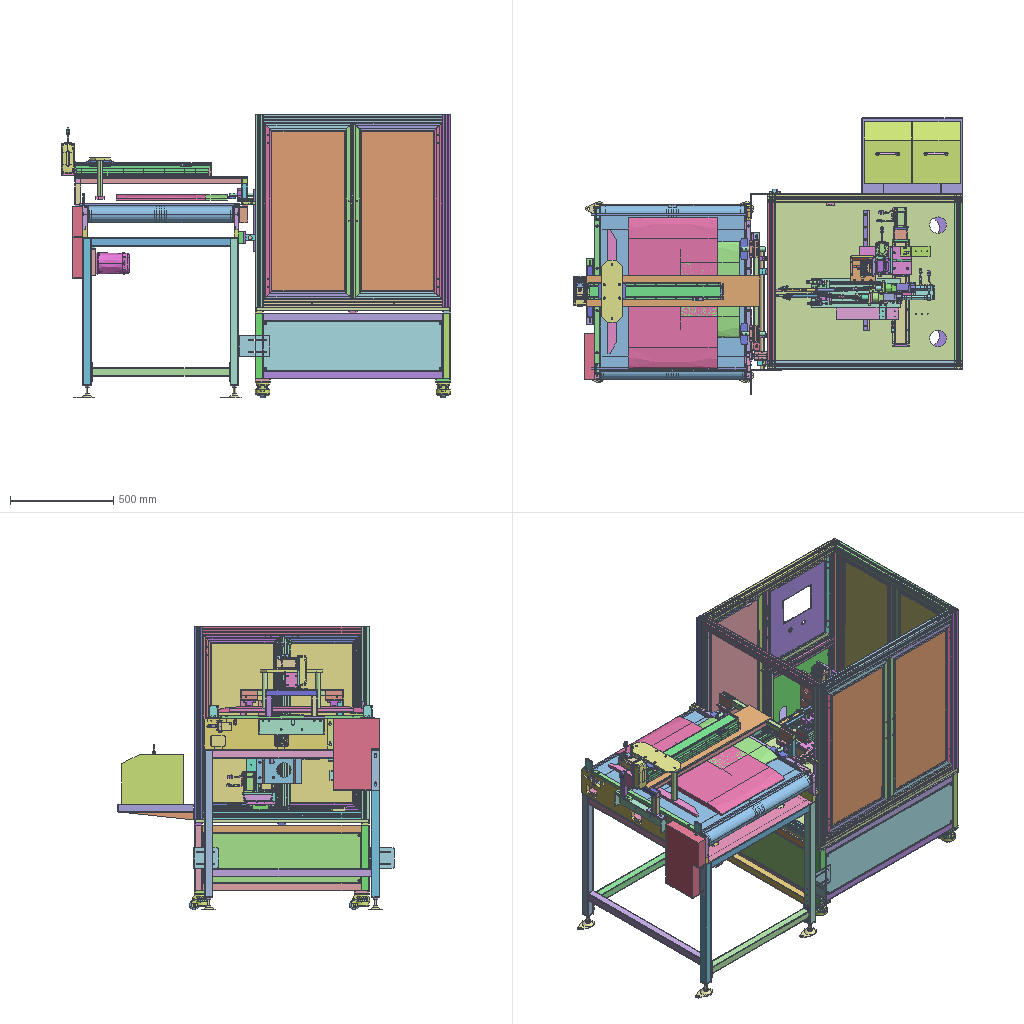Assembly | SolidWorks | 110 different items | 141 placed | box 1890 x 1340 x 1377 mm
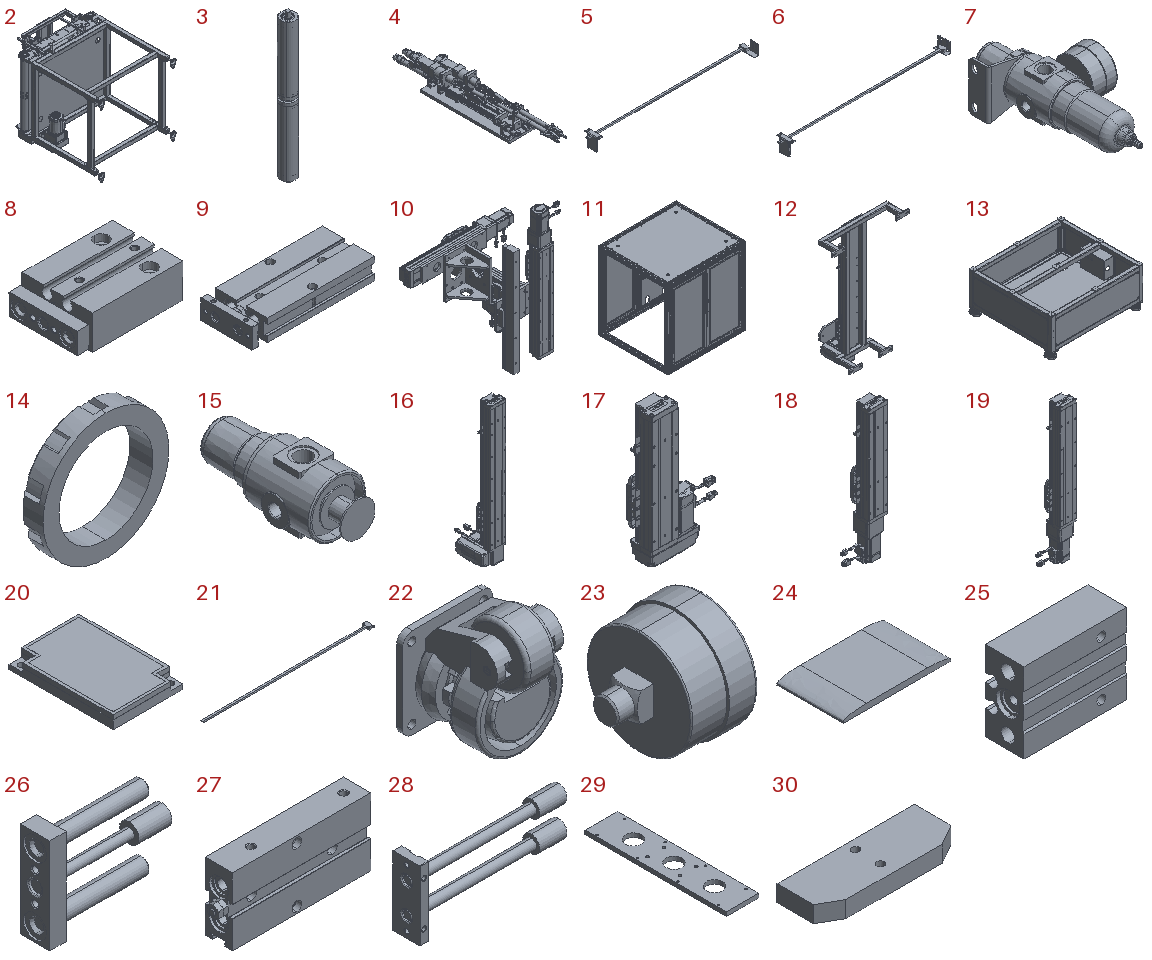Parts list (item | name | quantity | parent item | size | volume | features):
1 | (subassembly) | x1 | - | - | - | features Attribute 54, InContextFeatHolder 18
2 | (subassembly) | x1 | - | - | 25748774 mm3 | features ReferencePattern 2, CompositeCurve 1, MirrorCompFeat 1
3 | (subassembly) | x1 | in 2 | 76 x 76 x 755 mm | 913977 mm3 | features MirrorCompFeat 1
4 | (subassembly) | x1 | in 1 | - | 1977709 mm3 | -
5 | (subassembly) | x1 | in 2 | 779.985 x 90 x 92.8 mm | 90208 mm3 | -
6 | (subassembly) | x1 | in 2 | 779.985 x 68 x 92.8 mm | 89930 mm3 | -
7 | (subassembly) | x1 | in 13 | 87.334 x 158 x 50 mm | 129441 mm3 | features AEMSimFeature 1
8 | (subassembly) | x1 | in 2 | 44.5 x 30 x 14.5 mm | 15522 mm3 | features AEMSimFeature 1
9 | (subassembly) | x1 | in 2 | 98 x 42 x 17 mm | 52480 mm3 | features AEMSimFeature 1
10 | (subassembly) | x1 | in 1 | - | 10894817 mm3 | features InContextFeatHolder 20
11 | (subassembly) | x1 | - | - | 21354940 mm3 | -
12 | (subassembly) | x1 | in 2 | 570 x 381.182 x 905.5 mm | 5879539 mm3 | features ReferencePattern 4, InContextFeatHolder 2, MirrorCompFeat 1
13 | (subassembly) | x1 | - | 950 x 876 x 421.5 mm | 6731533 mm3 | features InContextFeatHolder 11, CompositeCurve 1
14 | - | x1 | in 7 | 38 x 7 x 38 mm | 3168 mm3 | features BaseBody 1
15 | - | x1 | in 7 | 40 x 98.3 x 40 mm | 76499 mm3 | features BaseBody 1
16 | - | x1 | in 12 | - | - | features BaseBody 15, RefSurface 8
17 | - | x1 | in 10 | - | - | features BaseBody 16, RefSurface 6
18 | - | x1 | in 10 | - | - | features BaseBody 14, RefSurface 8
19 | - | x2 | in 1, 10 | - | - | features BaseBody 14, RefSurface 8
20 | - | x2 | in 5, 6 | 40.3 x 59.9 x 7.5 mm | 17477 mm3 | features BaseBody 1
21 | - | x2 | in 5, 6 | 779.985 x 38.085 x 10.8 mm | 59248 mm3 | features BaseBody 1, ICE 1
22 | - | x4 | in 13 | 73 x 81.5 x 99 mm | 238657 mm3 | features BaseBody 4
23 | - | x1 | in 7 | 37.5 x 42 x 42 mm | 32291 mm3 | features BaseBody 1
24 | - | x1 | - | 465 x 285 x 25.029 mm | 3079068 mm3 | features Fillet 2, Extrusion 1
25 | - | x1 | in 8 | 38.5 x 14.5 x 30 mm | 12801 mm3 | features BaseBody 1
26 | - | x1 | in 8 | 38.7 x 9 x 29 mm | 2721 mm3 | features BaseBody 1
27 | - | x1 | in 9 | 93 x 17 x 42 mm | 43135 mm3 | features BaseBody 1
28 | - | x1 | in 9 | 90.1 x 16 x 41 mm | 9345 mm3 | features BaseBody 1
29 | - | x1 | in 10 | 80 x 350 x 10 mm | 238170 mm3 | features HoleWzd 2, Extrusion 1, ICE 1, LPattern 1
30 | - | x2 | in 12 | 100 x 35 x 12 mm | 39246 mm3 | features Chamfer 1, Extrusion 1, HoleWzd 1
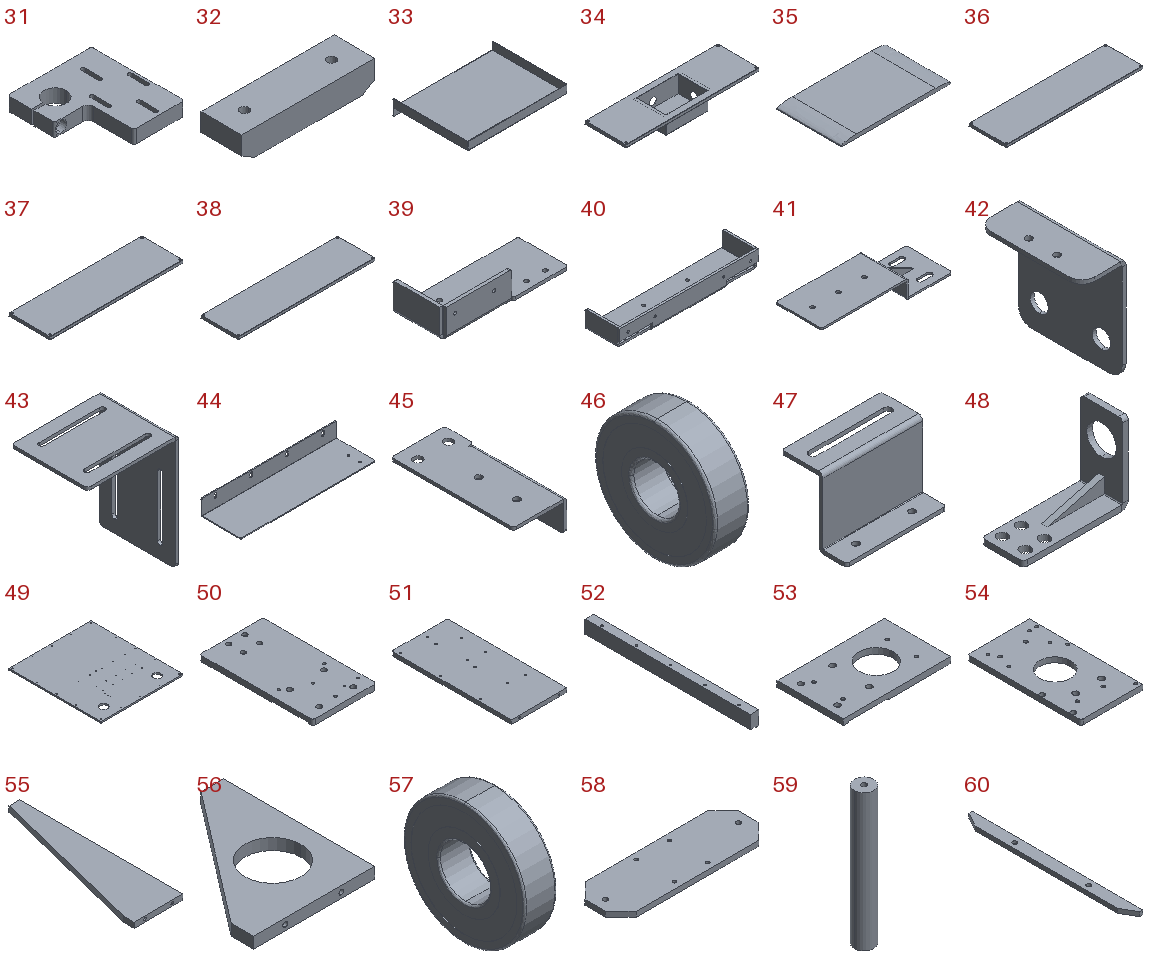31 | - | x1 | in 2 | 75 x 83 x 12 mm | 51875 mm3 | features ICE 4, HoleWzd 3, Fillet 2, LPattern 2, Extrusion 1, MoveFace 1
32 | - | x1 | in 2 | 52 x 16 x 10 mm | 7777 mm3 | features Chamfer 2, Extrusion 1, HoleWzd 1
33 | - | x1 | - | 490 x 370 x 77 mm | 765884 mm3 | features Gusset 2, EdgeFlange 1, Fillet 1, FlatPattern 1, HoleWzd 1, SMBaseFlange 1, SheetMetal 1
34 | - | x1 | in 13 | 768 x 238 x 101.5 mm | 482103 mm3 | features EdgeFlange 4, Cut 3, FlatPattern 2, HoleWzd 2, SMBaseFlange 2, SheetMetal 2, ICE 1
35 | - | x1 | - | 730 x 430 x 25.029 mm | 7503443 mm3 | features Fillet 2, Extrusion 1
36 | - | x1 | in 13 | 868 x 238 x 17.5 mm | 401918 mm3 | features EdgeFlange 2, Cut 1, FlatPattern 1, HoleWzd 1, SMBaseFlange 1, SheetMetal 1
37 | - | x1 | in 13 | 768 x 238 x 17.5 mm | 357698 mm3 | features EdgeFlange 2, Cut 1, FlatPattern 1, HoleWzd 1, SMBaseFlange 1, SheetMetal 1
38 | - | x1 | in 13 | 868 x 238 x 17.5 mm | 401918 mm3 | features EdgeFlange 2, Cut 1, FlatPattern 1, HoleWzd 1, SMBaseFlange 1, SheetMetal 1
39 | - | x1 | in 2 | 200 x 80 x 45 mm | 113530 mm3 | features HoleWzd 3, EdgeFlange 1, Fillet 1, FlatPattern 1, SMBaseFlange 1, SheetMetal 1
40 | - | x1 | in 2 | 320 x 80 x 40 mm | 194537 mm3 | features HoleWzd 3, MoveFace 2, EdgeFlange 1, Fillet 1, FlatPattern 1, ICE 1, MirrorPattern 1, SMBaseFlange 1, SheetMetal 1
41 | - | x1 | in 1 | 143 x 50 x 20 mm | 15978 mm3 | features EdgeFlange 2, Fillet 1, FlatPattern 1, Gusset 1, HoleWzd 1, ICE 1, SMBaseFlange 1, SheetMetal 1
42 | - | x1 | in 11 | 17 x 40 x 40 mm | 3135 mm3 | features HoleWzd 2, EdgeFlange 1, Fillet 1, FlatPattern 1, SMBaseFlange 1, SheetMetal 1
43 | - | x2 | - | 120 x 100 x 150 mm | 96309 mm3 | features ICE 2, EdgeFlange 1, Fillet 1, FlatPattern 1, SMBaseFlange 1, SheetMetal 1
44 | - | x1 | in 1 | 300 x 89 x 35 mm | 72285 mm3 | features EdgeFlange 1, Fillet 1, FlatPattern 1, HoleWzd 1, ICE 1, LPattern 1, SMBaseFlange 1, SheetMetal 1
45 | - | x1 | in 1 | 35 x 80 x 20 mm | 7504 mm3 | features HoleWzd 2, EdgeFlange 1, Fillet 1, FlatPattern 1, SMBaseFlange 1, SheetMetal 1
46 | - | x2 | in 3 | 15 x 52 x 52 mm | 19134 mm3 | features BaseBody 13
47 | - | x2 | in 12 | 80 x 52 x 56 mm | 23390 mm3 | features EdgeFlange 2, Fillet 1, FlatPattern 1, HoleWzd 1, ICE 1, SMBaseFlange 1, SheetMetal 1
48 | - | x1 | - | 55 x 22 x 42 mm | 5646 mm3 | features EdgeFlange 1, Fillet 1, FlatPattern 1, Gusset 1, HoleWzd 1, ICE 1, LPattern 1, SMBaseFlange 1, SheetMetal 1
49 | - | x1 | in 1 | 850 x 950 x 15 mm | 11946510 mm3 | features HoleWzd 5, Cut 1, Extrusion 1, Fillet 1, LPattern 1
50 | - | x1 | in 10 | 140 x 250 x 12 mm | 389185 mm3 | features HoleWzd 5, Extrusion 1, Fillet 1, ICE 1
51 | - | x1 | in 10 | 140 x 300 x 10 mm | 417191 mm3 | features HoleWzd 4, Extrusion 1, Fillet 1
52 | - | x1 | in 10 | 30 x 580 x 48 mm | 800287 mm3 | features HoleWzd 2, LPattern 2, Extrusion 1, ICE 1
53 | - | x1 | in 10 | 220 x 135 x 12 mm | 281633 mm3 | features HoleWzd 4, ICE 2, Extrusion 1
54 | - | x1 | in 10 | 120 x 220 x 10 mm | 227637 mm3 | features HoleWzd 5, Extrusion 1, Fillet 1, ICE 1
55 | - | x1 | in 10 | 90 x 300 x 10 mm | 171179 mm3 | features HoleWzd 2, Extrusion 1, ICE 1
56 | - | x4 | in 1, 10 | 108 x 135 x 10 mm | 74855 mm3 | features HoleWzd 2, ICE 2, Extrusion 1
57 | - | x2 | in 2 | 19 x 72 x 72 mm | 45746 mm3 | features BaseBody 14
58 | - | x1 | in 12 | 300 x 100 x 10 mm | 277705 mm3 | features HoleWzd 2, Chamfer 1, Extrusion 1
59 | - | x2 | in 2 | 25 x 25 x 176 mm | 84910 mm3 | features HoleWzd 2, Extrusion 1
60 | - | x1 | in 2 | 40 x 600 x 15 mm | 334405 mm3 | features Chamfer 1, Extrusion 1, HoleWzd 1
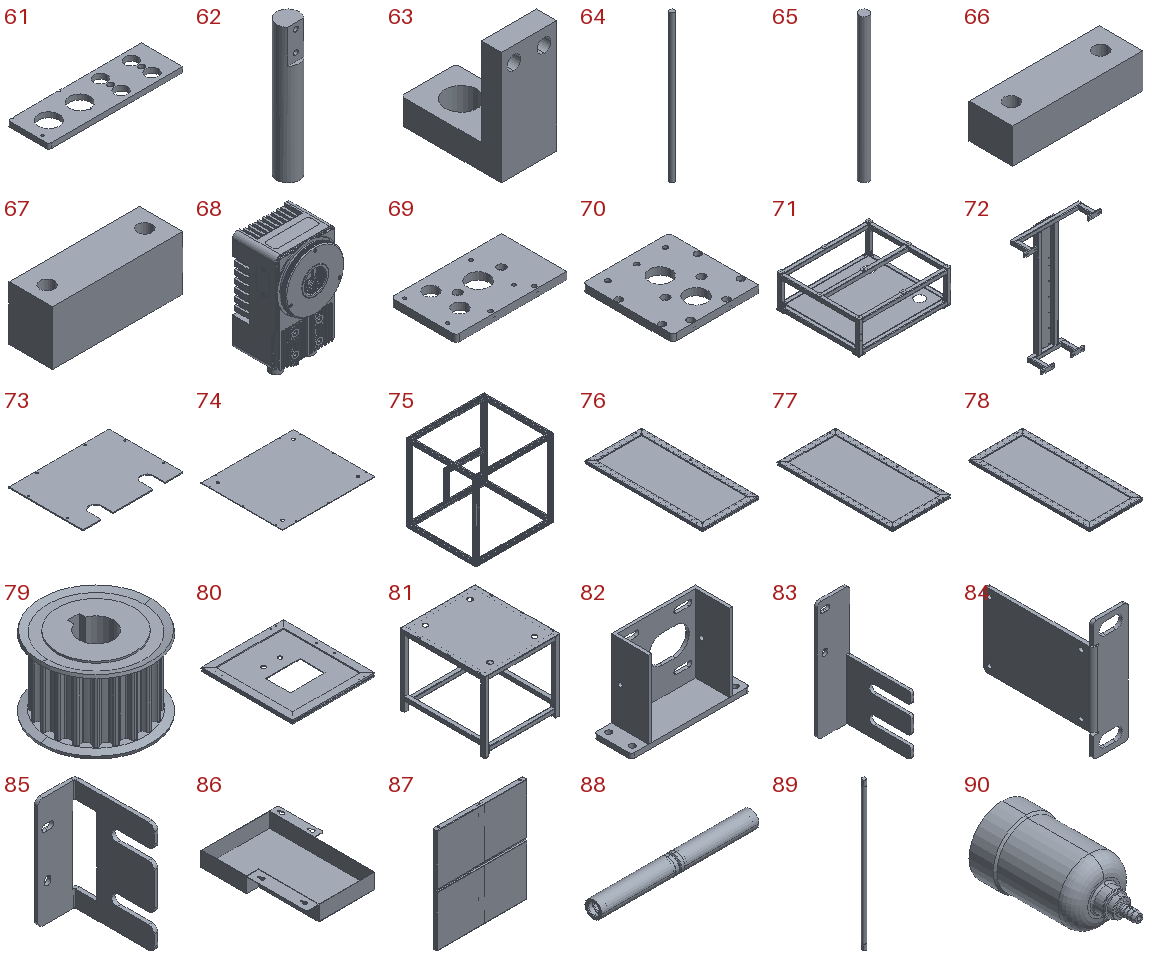61 | - | x1 | in 1 | 260 x 80 x 10 mm | 160429 mm3 | features HoleWzd 3, ICE 2, Extrusion 1, Fillet 1
62 | - | x2 | in 12 | 20 x 20 x 120 mm | 36039 mm3 | features HoleWzd 2, Extrusion 1, ICE 1
63 | - | x2 | - | 22 x 40 x 45 mm | 13243 mm3 | features BaseBody 1, ICE 1, MoveFace 1
64 | - | x1 | in 2 | 20 x 20 x 600 mm | 188496 mm3 | features Extrusion 1
65 | - | x2 | in 2 | 20 x 20 x 300 mm | 94248 mm3 | features Extrusion 1
66 | - | x1 | in 2 | 30 x 10 x 8 mm | 2124 mm3 | features Extrusion 1, HoleWzd 1
67 | - | x1 | in 2 | 60 x 20 x 25 mm | 28289 mm3 | features Extrusion 1, HoleWzd 1
68 | - | x1 | in 1 | - | - | features MBimport 1
69 | - | x1 | in 1 | 152 x 90 x 10 mm | 118972 mm3 | features HoleWzd 4, MoveFace 2, Extrusion 1, Fillet 1, ICE 1
70 | - | x1 | in 1 | 120 x 125 x 10 mm | 128886 mm3 | features HoleWzd 4, Fillet 2, ICE 2, Extrusion 1, MirrorPattern 1
71 | - | x1 | in 13 | 950 x 850 x 340 mm | 4003537 mm3 | features Fillet 10, Gusset 8, HoleWzd 8, WeldCornerFeat 8, MirrorSolid 4, ICE 3, 3DProfileFeature 1, EdgeFlange 1, FlatPattern 1, MirrorPattern 1, SMBaseFlange 1, SheetMetal 1, WeldMemberFeat 1, WeldmentFeature 1
72 | - | x1 | in 12 | 570 x 146 x 840 mm | 1678551 mm3 | features Fillet 4, ICE 4, 3DProfileFeature 1, EndCap 1, HoleWzd 1, MirrorPattern 1, WeldMemberFeat 1, WeldmentFeature 1
73 | - | x1 | in 11 | 416 x 308 x 4 mm | 483707 mm3 | features Fillet 2, HoleWzd 2, MirrorPattern 2, Extrusion 1, ICE 1
74 | - | x1 | in 11 | 868 x 768 x 4 mm | 2656781 mm3 | features MirrorPattern 4, HoleWzd 2, Extrusion 1, Fillet 1, ICE 1
75 | - | x1 | in 11 | 950 x 850 x 940 mm | 5673815 mm3 | features WeldCornerFeat 8, 3DProfileFeature 5, HoleWzd 4, ICE 1, WeldMemberFeat 1, WeldmentFeature 1
76 | - | x1 | in 11 | 407 x 856 x 20 mm | 2220771 mm3 | features HoleWzd 3, ICE 1, WeldMemberFeat 1, WeldmentFeature 1
77 | - | x2 | in 11 | 432 x 856 x 20 mm | 2324012 mm3 | features HoleWzd 3, ICE 1, WeldMemberFeat 1, WeldmentFeature 1
78 | - | x2 | in 11 | 382 x 856 x 20 mm | 2117530 mm3 | features HoleWzd 3, ICE 1, WeldMemberFeat 1, WeldmentFeature 1
79 | - | x2 | in 2 | 58 x 58 x 38.085 mm | 55625 mm3 | features BaseBody 1, ICE 1
80 | - | x1 | in 11 | 456 x 508 x 20 mm | 1433646 mm3 | features HoleWzd 3, ICE 3, WeldMemberFeat 1, WeldmentFeature 1
81 | - | x1 | in 2 | 755 x 850 x 720 mm | 5913243 mm3 | features ICE 14, Fillet 3, Cut 1, Extrusion 1, LPattern 1
82 | - | x1 | in 2 | 190 x 60 x 132 mm | 223205 mm3 | features ICE 3, Cut 1, Extrusion 1, Fillet 1
83 | - | x1 | in 5 | 22 x 45 x 80 mm | 6161 mm3 | features ICE 4, Fillet 2, ExtruThin 1, FlatPattern 1, FlattenBends 1, ProcessBends 1, SheetMetal 1
84 | - | x2 | in 5, 6 | 20 x 62 x 68 mm | 7322 mm3 | features ICE 4, Cut 1, ExtruThin 1, Fillet 1, FlatPattern 1, FlattenBends 1, ProcessBends 1, SheetMetal 1
85 | - | x1 | in 6 | 22 x 45 x 60 mm | 5883 mm3 | features Fillet 2, ICE 2, Cut 1, ExtruThin 1, FlatPattern 1, FlattenBends 1, ProcessBends 1, SheetMetal 1
86 | - | x1 | in 2 | 255 x 350 x 50 mm | 207064 mm3 | features Fillet 2, ICE 2, Cut 1, Extrusion 1, Shell 1
87 | - | x1 | in 2 | 620 x 30 x 714 mm | 1123821 mm3 | features ICE 4, BossThin 2, Extrusion 1, Fillet 1, FlatPattern 1, FlattenBends 1, LPattern 1, ProcessBends 1, Rip 1, SheetMetal 1, Shell 1
88 | - | x1 | in 3 | 705 x 76 x 76 mm | 640493 mm3 | features ICE 3, RevCut 2, Revolution 2, MirrorPattern 1
89 | - | x1 | in 3 | 20 x 20 x 755 mm | 235219 mm3 | features ICE 2, Extrusion 1, MirrorPattern 1
90 | - | x1 | in 7 | 35.6 x 74 x 35.6 mm | 13537 mm3 | features BaseBody 1
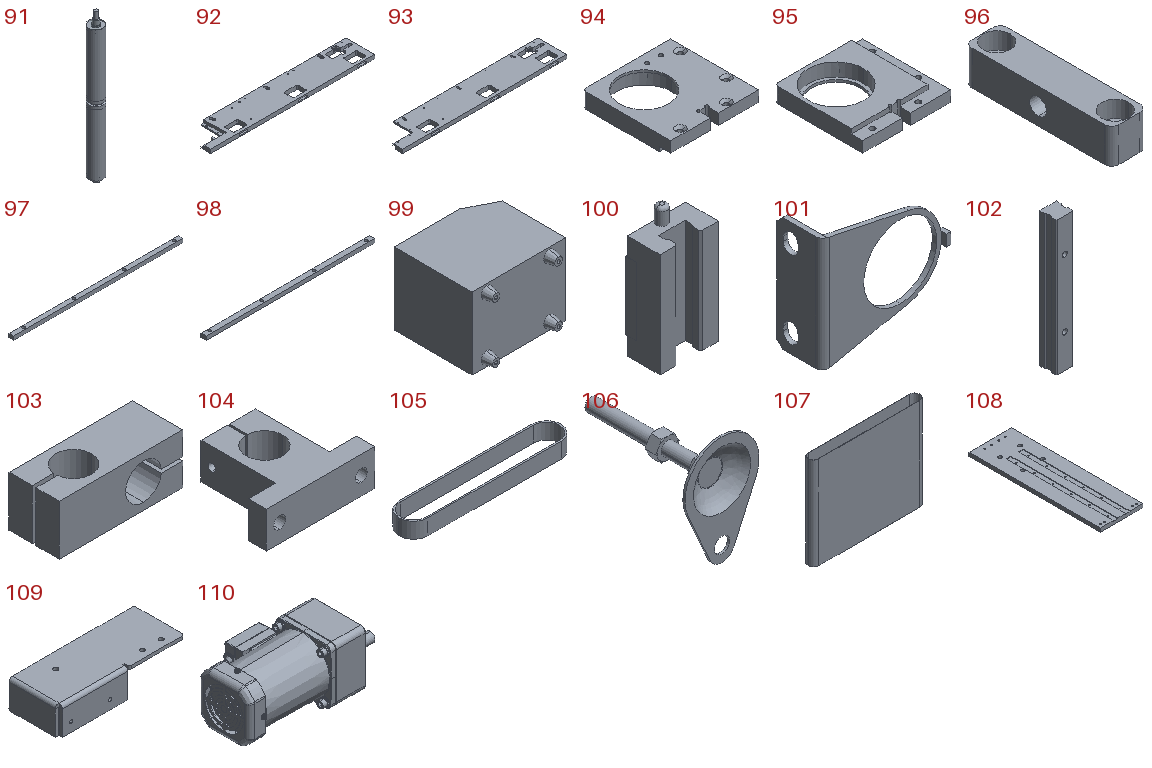91 | - | x1 | in 2 | 76 x 76 x 795 mm | 1220082 mm3 | features ICE 9, Extrusion 1, RevCut 1, Revolution 1
92 | - | x1 | in 2 | 850 x 150 x 20 mm | 1984995 mm3 | features HoleWzd 7, ICE 6, Fillet 4, Cut 1, Extrusion 1, LPattern 1
93 | - | x1 | in 2 | 850 x 150 x 20 mm | 1984995 mm3 | features MirrorStock 1
94 | - | x1 | in 2 | 115 x 115 x 20 mm | 159742 mm3 | features ICE 5, HoleWzd 3, Extrusion 1, Fillet 1
95 | - | x1 | in 2 | 115 x 115 x 20 mm | 159742 mm3 | features MirrorStock 1
96 | - | x2 | in 2 | 14.5 x 59.5 x 14 mm | 9659 mm3 | features HoleWzd 2, Extrusion 1, Fillet 1
97 | - | x1 | in 2 | 690 x 20 x 15 mm | 203293 mm3 | features Extrusion 1, HoleWzd 1, ICE 1
98 | - | x1 | in 2 | 665 x 20 x 15 mm | 195793 mm3 | features Extrusion 1, HoleWzd 1
99 | - | x2 | - | - | - | features BaseBody 11, RefSurface 2
100 | - | x1 | in 10 | 44 x 25.4 x 89.5 mm | 65459 mm3 | features ICE 7, Extrusion 1, Fillet 1
101 | - | x1 | in 7 | 54 x 22.2 x 50 mm | 3948 mm3 | features BaseBody 1
102 | - | x1 | in 10 | 15 x 15 x 120 mm | 24720 mm3 | features MoveFace 2, Chamfer 1, Extrusion 1, LPattern 1, RevCut 1
103 | - | x2 | in 2 | 69 x 28 x 28 mm | 35157 mm3 | features ICE 2, Extrusion 1
104 | - | x4 | in 2, 12 | 60 x 51 x 20 mm | 28604 mm3 | features HoleWzd 3, Extrusion 1, RefAxis 1
105 | - | x1 | in 2 | 312 x 56 x 30 mm | 61065 mm3 | features ExtruThin 1
106 | - | x4 | in 2 | 68 x 121 x 100 mm | 26277 mm3 | features BaseBody 2
107 | - | x1 | in 2 | 845 x 80 x 700 mm | 2508235 mm3 | features ExtruThin 1, ICE 1
108 | - | x1 | - | 140 x 430 x 12 mm | 670240 mm3 | features BaseBody 1, Fillet 1, HoleWzd 1, ICE 1
109 | - | x1 | in 2 | 200 x 80 x 45 mm | 113530 mm3 | features MirrorStock 1
110 | - | x1 | in 2 | 261 x 143.386 x 105.972 mm | 1074405 mm3 | features BaseBody 4
Mates (type | each side: item.copy, entity, surface, feature):
In the top assembly
Coincident | 71.1 face plane Boss-Extrude 1 | 49.1 face plane Boss-Extrude 1
Coincident | 71.1 face plane Cold-Formed Square Hollow Tube gb∕t6728-2002 40 X 40 X 2(1) | 49.1 face plane Boss-Extrude 1 | 2 times
Coincident | 49.1 face plane Boss-Extrude 1 | 75.1 face plane Industrial Aluminium Profile 40 X 40GE X R0.3(1) | 3 times
Coincident | assembly face | 106.1 face plane HI_WAN11-D100-M12-L100-001-1-solid1
DistanceDim | 81.1 face plane Boss-Extrude 5 | 71.1 face plane Cold-Formed Square Hollow Tube gb∕t6728-2002 40 X 40 X 2(1)
Parallel | 75.1 face plane Industrial Aluminium Profile 40 X 40GE X R0.3(1) | 99.1 face plane
Coincident | 75.1 face plane Industrial Aluminium Profile 40 X 40GE X R0.3(1) | 99.1 face plane
Coincident | 99.1 face plane | 99.2 face plane | 2 times
DistanceDim | 99.2 face plane | 99.1 face plane
Coincident | 75.1 face plane Industrial Aluminium Profile 40 X 40GE X R0.3(1) | 33.1 face plane Edge-Flange 1 | 2 times
Coincident | 49.1 face plane Boss-Extrude 1 | 33.1 face plane Edge-Flange 1
Width | 33.1 face plane Edge-Flange 1 | 33.1 face plane Edge-Flange 1 | 99.1 face plane | 99.2 face plane
DistanceDim | 99.1 face plane | 33.1 face plane Edge-Flange 1
DistanceDim | 71.1 face plane Cold-Formed Square Hollow Tube gb∕t6728-2002 40 X 40 X 2(1) | 81.1 face plane Boss-Extrude 3
DistanceDim | 107.1 face plane Extrude-Thin 1 | 24.1 face plane Boss-Extrude 1
Tangent | 22.1 face cylinder GD-60F Foot Master Caster [GD-60F].step-1/HI_CGR51-60-U-001.step-1-solid1 | 106.1 face plane HI_WAN11-D100-M12-L100-001-1-solid1
Parallel | 86.1 face plane Boss-Extrude 1 | 24.1 face plane Boss-Extrude 1
DistanceDim | 107.1 face plane Extrude-Thin 1 | 35.1 face plane Boss-Extrude 1
Width | 97.1 face plane Boss-Extrude 1 | 98.1 face plane Boss-Extrude 1 | 35.1 face plane Boss-Extrude 1 | 35.1 face plane Boss-Extrude 1
Coincident | 71.1 face plane Cold-Formed Square Hollow Tube gb∕t6728-2002 40 X 40 X 2(1) | 43.1 face plane Edge-Flange 1
Coincident | 81.1 face plane Boss-Extrude 3 | 43.1 face plane Base-Flange 1
DistanceDim | 43.1 face plane Base-Flange 1 | 71.1 face plane Cold-Formed Square Hollow Tube gb∕t6728-2002 40 X 40 X 2(1)
Coincident | 71.1 face plane Cold-Formed Square Hollow Tube gb∕t6728-2002 40 X 40 X 2(1) | 43.2 face plane Edge-Flange 1
Coincident | 81.1 face plane Boss-Extrude 3 | 43.2 face plane Base-Flange 1
Coincident | 43.1 face plane Base-Flange 1 | 43.2 face plane Edge-Flange 1
In subassembly 1
Coincident | 49.2 face plane Boss-Extrude 1 | 19.1 face plane
Width | 108.1 face plane Import 1 | 108.1 face plane Import 1 | 18.1 face plane | 18.1 face plane
Coincident | 18.1 face plane | 108.1 face plane Import 1
DistanceDim | 19.1 face plane | 49.2 face plane Boss-Extrude 1 | 2 times
Coincident | 54.1 face plane Boss-Extrude 1 | 61.1 face plane Boss-Extrude 1 | 2 times
Coincident | 68.1 face plane 69x62x117-X86-3DK-3D-V2.0.stp<1> | 61.1 face plane Boss-Extrude 1
DistanceDim | 61.1 face plane Boss-Extrude 1 | 54.1 face plane Boss-Extrude 1
Coincident | 54.1 face plane Boss-Extrude 1 | 56.1 face plane Boss-Extrude 1
Coincident | 61.1 face plane Boss-Extrude 1 | 56.1 face plane Boss-Extrude 1
Width | 61.1 face plane Boss-Extrude 1 | 61.1 face plane Boss-Extrude 1 | 56.1 face plane Boss-Extrude 1 | 56.1 face plane Boss-Extrude 1
Coincident | 18.1 face plane | 108.1 face plane Cut-Extrude 1
Coincident | 50.1 face plane Boss-Extrude 1 | 41.1 face plane Base-Flange 1 | 2 times
Coincident | 50.1 face plane Boss-Extrude 1 | 41.1 face plane Edge-Flange 1
Coincident | 29.1 face plane Boss-Extrude 1 | 44.1 face plane Edge-Flange 1 | 3 times
Coincident | 108.1 face plane Import 1 | 45.1 face plane Base-Flange 1
Coincident | 108.1 face plane Import 1 | 45.1 face plane Edge-Flange 1
Coincident | 49.2 face plane Boss-Extrude 1 | 19.2 face plane
Concentric | 49.2 face cylinder LPattern 1 | 19.2 face cylinder | 2 times
DistanceDim | 54.1 face plane Boss-Extrude 1 | 70.1 face plane Boss-Extrude 1
Coincident | 54.1 face plane Boss-Extrude 1 | 70.1 face plane Boss-Extrude 1
Coincident | 108.1 face plane Import 1 | 70.1 face plane Boss-Extrude 1
Coincident | 70.1 face plane Boss-Extrude 1 | 69.1 face plane Boss-Extrude 1
Parallel | 70.1 face plane Boss-Extrude 1 | 69.1 face plane Boss-Extrude 1
Concentric | 70.1 face cylinder Mirror 1 | 69.1 face cylinder M5 Tapped Hole 1
Coincident | 68.1 face plane 69x62x117-X86-3DK-3D-V2.0.stp<1> | 69.1 face plane Boss-Extrude 1
Coincident | 70.1 face plane Boss-Extrude 1 | 56.2 face plane Boss-Extrude 1 | 2 times
Coincident | 69.1 face plane Boss-Extrude 1 | 56.2 face plane Boss-Extrude 1
Concentric | 68.1 face cylinder 69x62x117-X86-3DK-3D-V2.0.stp<1> | 69.1 face cylinder Hole Size (% for) Socket Head Cap Screw Type 2
In subassembly 10
Coincident | 50.2 face plane Boss-Extrude 1 | 51.1 face plane Boss-Extrude 1 | 2 times
DistanceDim | 51.1 face plane Boss-Extrude 1 | 50.2 face plane Boss-Extrude 1
Coincident | 51.1 face plane Boss-Extrude 1 | 17.1 face plane | 2 times
Coincident | 50.2 face plane Boss-Extrude 1 | 17.1 face plane
Coincident | 52.1 face plane Boss-Extrude 1 | 102.1 face plane Boss-Extrude 1
Coincident | 52.1 face plane Cut-Extrude 1 | 102.1 face plane Boss-Extrude 1 | 2 times
Coincident | 102.1 face plane Boss-Extrude 1 | 100.1 face plane Boss-Extrude 1 | 2 times
Width | 50.2 face plane Boss-Extrude 1 | 50.2 face plane Boss-Extrude 1 | 100.1 face plane Boss-Extrude 1 | 100.1 face plane Boss-Extrude 1
Coincident | 53.1 face plane Boss-Extrude 1 | 54.2 face plane Boss-Extrude 1 | 3 times
Parallel | 53.1 face plane Boss-Extrude 1 | 54.2 face plane Boss-Extrude 1
Coincident | 54.2 face plane Boss-Extrude 1 | 29.2 face plane Boss-Extrude 1 | 2 times
Width | 29.2 face plane Boss-Extrude 1 | 29.2 face plane Boss-Extrude 1 | 54.2 face plane Boss-Extrude 1 | 54.2 face plane Boss-Extrude 1
Coincident | 29.2 face plane Boss-Extrude 1 | 18.2 face plane | 3 times
DistanceDim | 53.1 face plane Boss-Extrude 1 | 17.1 face plane
Width | 53.1 face plane Boss-Extrude 1 | 54.2 face plane Boss-Extrude 1 | 17.1 face plane | 17.1 face plane
Coincident | 50.2 face plane Boss-Extrude 1 | 55.1 face plane Boss-Extrude 1
Coincident | 51.1 face plane Boss-Extrude 1 | 55.1 face plane Boss-Extrude 1
Width | 50.2 face plane Boss-Extrude 1 | 50.2 face plane Boss-Extrude 1 | 55.1 face plane Boss-Extrude 1 | 55.1 face plane Boss-Extrude 1
Coincident | 53.1 face plane Boss-Extrude 1 | 56.1 face plane Boss-Extrude 1
Coincident | 54.2 face plane Boss-Extrude 1 | 56.1 face plane Boss-Extrude 1
DistanceDim | 56.1 face plane Boss-Extrude 1 | 53.1 face plane Boss-Extrude 1
Coincident | 53.1 face plane Boss-Extrude 1 | 56.3 face plane Boss-Extrude 1
Coincident | 54.2 face plane Boss-Extrude 1 | 56.3 face plane Boss-Extrude 1
DistanceDim | 56.3 face plane Boss-Extrude 1 | 54.2 face plane Boss-Extrude 1
Coincident | 17.1 face plane | 53.1 face plane Cut-Extrude 1
Coincident | 19.2 face plane | 50.2 face plane Cut-Extrude 1
Width | 19.2 face plane | 19.2 face plane | 50.2 face plane Cut-Extrude 1 | 50.2 face plane Cut-Extrude 1
DistanceDim | 19.2 face plane | 52.1 face plane Boss-Extrude 1
Coincident | 19.2 face plane | 52.1 face plane Boss-Extrude 1
In subassembly 13
Coincident | 71.2 face plane Boss-Extrude 2 | 22.2 face plane GD-60F Foot Master Caster [GD-60F].step-1/HI_CGR51-60-U-003.step-1-solid1
Width | 22.2 face plane GD-60F Foot Master Caster [GD-60F].step-1/HI_CGR51-60-U-003.step-1-solid1 | 22.2 face plane GD-60F Foot Master Caster [GD-60F].step-1/HI_CGR51-60-U-003.step-1-solid1 | 71.2 face plane Boss-Extrude 2 | 71.2 face plane Boss-Extrude 2 | 2 times
Coincident | 71.2 face plane Mirror 2 | 22.3 face plane GD-60F Foot Master Caster [GD-60F].step-1/HI_CGR51-60-U-003.step-1-solid1 | 3 times
Coincident | 71.2 face plane Mirror 2 | 22.4 face plane GD-60F Foot Master Caster [GD-60F].step-1/HI_CGR51-60-U-003.step-1-solid1
Concentric | 71.2 face cylinder Mirror 2 | 22.4 face cylinder GD-60F Foot Master Caster [GD-60F].step-1/HI_CGR51-60-U-003.step-1-solid1
Parallel | 71.2 face plane Mirror 2 | 22.4 face plane GD-60F Foot Master Caster [GD-60F].step-1/HI_CGR51-60-U-003.step-1-solid1
Concentric | 71.2 edge | 22.5 face cylinder GD-60F Foot Master Caster [GD-60F].step-1/HI_CGR51-60-U-003.step-1-solid1
Coincident | 71.2 face plane Mirror 1 | 22.5 face plane GD-60F Foot Master Caster [GD-60F].step-1/HI_CGR51-60-U-003.step-1-solid1
Parallel | 71.2 face plane Mirror 1 | 22.5 face plane GD-60F Foot Master Caster [GD-60F].step-1/HI_CGR51-60-U-003.step-1-solid1
Coincident | 71.2 face plane Cold-Formed Square Hollow Tube gb∕t6728-2002 40 X 40 X 2(1) | 34.1 face plane Base-Flange 1
Width | 71.2 face plane Cold-Formed Square Hollow Tube gb∕t6728-2002 40 X 40 X 2(1) | 71.2 face plane Cold-Formed Square Hollow Tube gb∕t6728-2002 40 X 40 X 2(1) | 34.1 face plane Edge-Flange 1 | 34.1 face plane Edge-Flange 1 | 2 times
Coincident | 71.2 face plane Cold-Formed Square Hollow Tube gb∕t6728-2002 40 X 40 X 2(1) | 37.1 face plane Base-Flange 1
Width | 71.2 face plane Cold-Formed Square Hollow Tube gb∕t6728-2002 40 X 40 X 2(1) | 71.2 face plane Cold-Formed Square Hollow Tube gb∕t6728-2002 40 X 40 X 2(1) | 37.1 face plane Edge-Flange 1 | 37.1 face plane Edge-Flange 1 | 2 times
Coincident | 71.2 face plane Cold-Formed Square Hollow Tube gb∕t6728-2002 40 X 40 X 2(1) | 36.1 face plane Base-Flange 1
Width | 71.2 face plane Cold-Formed Square Hollow Tube gb∕t6728-2002 40 X 40 X 2(1) | 71.2 face plane Cold-Formed Square Hollow Tube gb∕t6728-2002 40 X 40 X 2(1) | 36.1 face plane Edge-Flange 1 | 36.1 face plane Edge-Flange 1 | 2 times
Coincident | 71.2 face plane Cold-Formed Square Hollow Tube gb∕t6728-2002 40 X 40 X 2(1) | 38.1 face plane Base-Flange 1
Width | 71.2 face plane Cold-Formed Square Hollow Tube gb∕t6728-2002 40 X 40 X 2(1) | 71.2 face plane Cold-Formed Square Hollow Tube gb∕t6728-2002 40 X 40 X 2(1) | 38.1 face plane Edge-Flange 1 | 38.1 face plane Edge-Flange 1 | 2 times
Coincident | 34.1 face plane Base-Flange 2 | 101.1 face plane AFR2000 Fl
DistanceDim | 15.1 face plane AFR2000 Sw | 34.1 face plane Edge-Flange 3
DistanceDim | 101.1 face plane AFR2000 Fl | 34.1 face plane Edge-Flange 3
In subassembly 11
DistanceDim | 76.1 face plane Aluminium Profile 2040A(1) | 75.2 face plane Industrial Aluminium Profile 40 X 40GE X R0.3(1)
Width | 76.1 face plane Aluminium Profile 2040A(1) | 76.1 face plane Aluminium Profile 2040A(1) | 75.2 face plane Industrial Aluminium Profile 40 X 40GE X R0.3(1) | 75.2 face plane Industrial Aluminium Profile 40 X 40GE X R0.3(1)
Coincident | 75.2 face plane Industrial Aluminium Profile 40 X 40GE X R0.3(1) | 77.1 face plane Aluminium Profile 2040A(1)
Coincident | 76.1 face plane Aluminium Profile 2040A(1) | 77.1 face plane Aluminium Profile 2040A(1)
DistanceDim | 77.1 face plane Aluminium Profile 2040A(1) | 75.2 face plane Industrial Aluminium Profile 40 X 40GE X R0.3(1)
Coincident | 77.1 face plane Aluminium Profile 2040A(1) | 77.2 face plane Aluminium Profile 2040A(1) | 2 times
DistanceDim | 77.2 face plane Aluminium Profile 2040A(1) | 75.2 face plane Industrial Aluminium Profile 40 X 40GE X R0.3(1)
Coincident | 75.2 face plane Industrial Aluminium Profile 40 X 40GE X R0.3(1) | 78.1 face plane Aluminium Profile 2040A(1)
Width | 78.1 face plane Aluminium Profile 2040A(1) | 78.1 face plane Aluminium Profile 2040A(1) | 75.2 face plane Industrial Aluminium Profile 40 X 40GE X R0.3(1) | 75.2 face plane Industrial Aluminium Profile 40 X 40GE X R0.3(1)
DistanceDim | 78.1 face plane Aluminium Profile 2040A(1) | 75.2 face plane Industrial Aluminium Profile 40 X 40GE X R0.3(1)
Coincident | 75.2 face plane Industrial Aluminium Profile 40 X 40GE X R0.3(1) | 78.2 face plane Aluminium Profile 2040A(1)
Width | 78.2 face plane Aluminium Profile 2040A(1) | 78.2 face plane Aluminium Profile 2040A(1) | 75.2 face plane Industrial Aluminium Profile 40 X 40GE X R0.3(1) | 75.2 face plane Industrial Aluminium Profile 40 X 40GE X R0.3(1)
DistanceDim | 78.2 face plane Aluminium Profile 2040A(1) | 75.2 face plane Industrial Aluminium Profile 40 X 40GE X R0.3(1)
Coincident | 75.2 face plane Industrial Aluminium Profile 40 X 40GE X R0.3(1) | 76.1 face plane Aluminium Profile 2040A(1)
Coincident | 75.2 face plane Industrial Aluminium Profile 40 X 40GE X R0.3(1) | 80.1 face plane Aluminium Profile 2040A(1)
Width | 75.2 face plane Industrial Aluminium Profile 40 X 40GE X R0.3(1) | 75.2 face plane Industrial Aluminium Profile 40 X 40GE X R0.3(1) | 80.1 face plane Aluminium Profile 2040A(1) | 80.1 face plane Aluminium Profile 2040A(1)
DistanceDim | 80.1 face plane Aluminium Profile 2040A(1) | 75.2 face plane Industrial Aluminium Profile 40 X 40GE X R0.3(1)
Coincident | 75.2 face plane Industrial Aluminium Profile 40 X 40GE X R0.3(1) | 73.1 face plane Boss-Extrude 1
Width | 75.2 face plane Industrial Aluminium Profile 40 X 40GE X R0.3(1) | 75.2 face plane Industrial Aluminium Profile 40 X 40GE X R0.3(1) | 73.1 face plane Boss-Extrude 1 | 73.1 face plane Boss-Extrude 1 | 2 times
Coincident | 75.2 face plane Industrial Aluminium Profile 40 X 40GE X R0.3(1) | 74.1 face plane Boss-Extrude 1
Width | 75.2 face plane Industrial Aluminium Profile 40 X 40GE X R0.3(1) | 75.2 face plane Industrial Aluminium Profile 40 X 40GE X R0.3(1) | 74.1 face plane Boss-Extrude 1 | 74.1 face plane Boss-Extrude 1 | 2 times
Coincident | 75.2 face plane Industrial Aluminium Profile 40 X 40GE X R0.3(1) | 42.1 face plane Edge-Flange 1
DistanceDim | 42.1 face plane Base-Flange 1 | 75.2 face plane Industrial Aluminium Profile 40 X 40GE X R0.3(1)
In subassembly 2
Coincident | 92.1 face plane Cut-Extrude 2 | 94.1 face plane Cut-Extrude 1
Coincident | 92.1 face plane Cut-Extrude 2 | 94.1 face plane Boss-Extrude 1 | 2 times
Coincident | 94.1 face plane Cut-Extrude 3 | 57.1 face plane 1-1-solid1
Concentric | 94.1 face cylinder Cut-Extrude 3 | 57.1 face cylinder 1-1-solid1
Coincident | 92.1 face plane Cut-Extrude 4 | 96.1 face plane Boss-Extrude 1
Concentric | 92.1 face cylinder M6 Tapped Hole 2 | 96.1 face cylinder Hole Size (% for) Socket Head Cap Screw Type 2
Concentric | 107.2 face cylinder Extrude-Thin 1 | 57.1 face cylinder 3-1-solid1
Parallel | 107.2 face plane Extrude-Thin 1 | 92.1 face plane Boss-Extrude 1
DistanceDim | 107.2 edge | 92.1 face plane Boss-Extrude 1
Coincident | 92.1 face plane Boss-Extrude 1 | 89.1 face plane Boss-Extrude 1
Concentric | 57.1 face cylinder 3-1-solid1 | 91.1 face cylinder Cut-Extrude 3
Coincident | 92.1 face plane Boss-Extrude 1 | 87.1 face plane Boss-Extrude 1
Coincident | 107.2 face plane Extrude-Thin 1 | 87.1 face plane Boss-Extrude 1
Concentric | 107.2 face cylinder Extrude-Thin 1 | 88.1 face cylinder Revolve 1
Coincident | 94.1 face plane Boss-Extrude 1 | 91.1 face plane Boss-Extrude 4
Coincident | 95.1 face plane | 57.2 face plane 1-1-solid1
Concentric | 95.1 face cylinder | 57.2 face cylinder 1-1-solid1
Coincident | 93.1 face plane | 96.2 face plane Boss-Extrude 1
Concentric | 93.1 face cylinder | 96.2 face cylinder Hole Size (% for) Socket Head Cap Screw Type 2 | 2 times
Concentric | 91.1 face cylinder Cut-Extrude 5 | 105.1 face cylinder Extrude-Thin 1
Coincident | 105.1 face plane Extrude-Thin 1 | 79.1 face plane Import 1
DistanceDim | 79.1 face plane Import 1 | 95.1 face plane
Coincident | 93.1 face plane | 81.2 face plane Boss-Extrude 1 | 3 times
Concentric | 81.2 face cylinder Boss-Extrude 6 | 106.2 face cylinder HI_WAN11-D100-M12-L100-001-1-solid1
Coincident | 81.2 face plane Boss-Extrude 6 | 106.2 face plane HI_WAN11-D100-M12-L100-002-1-solid1
Concentric | 81.2 face cylinder Boss-Extrude 6 | 106.3 face cylinder HI_WAN11-D100-M12-L100-001-1-solid1
Coincident | 81.2 face plane Boss-Extrude 6 | 106.3 face plane HI_WAN11-D100-M12-L100-002-1-solid1
Concentric | 81.2 face cylinder Boss-Extrude 6 | 106.4 face cylinder HI_WAN11-D100-M12-L100-001-1-solid1
Coincident | 81.2 face plane Boss-Extrude 6 | 106.4 face plane HI_WAN11-D100-M12-L100-002-1-solid1
Concentric | 81.2 face cylinder Boss-Extrude 6 | 106.5 face cylinder HI_WAN11-D100-M12-L100-001-1-solid1
Coincident | 81.2 face plane Boss-Extrude 6 | 106.5 face plane HI_WAN11-D100-M12-L100-002-1-solid1
Concentric | 110.1 face cylinder 100GF-H-18-1-solid1 | 79.2 face cylinder Cut-Extrude 1
Coincident | 79.1 face plane Import 1 | 79.2 face plane Import 1
Parallel | 110.1 face plane 100GF-H-18-1-solid2 | 81.2 face plane Boss-Extrude 5
Concentric | 110.1 face cylinder 100GF-H-18-1-solid1 | 105.1 face cylinder Extrude-Thin 1
Coincident | 81.2 face plane Boss-Extrude 7 | 82.1 face plane Boss-Extrude 1 | 3 times
Coincident | 110.1 face plane 100GF-H-18-1-solid2 | 82.1 face plane Boss-Extrude 2
Coincident | 92.1 face plane Boss-Extrude 1 | 83.1 face plane Extrude-Thin 1
DistanceDim | 94.1 face plane Boss-Extrude 1 | 83.1 face plane Extrude-Thin 1
Coincident | 92.1 face plane Boss-Extrude 1 | 85.1 face plane Extrude-Thin 1
DistanceDim | 85.1 face plane Extrude-Thin 1 | 92.1 face plane Boss-Extrude 1
Coincident | 92.1 face plane Boss-Extrude 1 | 98.2 face plane Boss-Extrude 1 | 2 times
Coincident | 93.1 face plane | 97.2 face plane Boss-Extrude 1
Concentric | 93.1 face cylinder | 97.2 face cylinder Hole Size (% for) Socket Head Cap Screw Type 1 | 2 times
Coincident | 81.2 face plane Boss-Extrude 5 | 86.2 face plane Boss-Extrude 1
Coincident | 81.2 face plane Boss-Extrude 3 | 86.2 face plane Boss-Extrude 1
Coincident | 95.1 face plane | 86.2 face plane Boss-Extrude 1
Coincident | 92.1 face plane Boss-Extrude 1 | 39.1 face plane Base-Flange 1
Coincident | 92.1 face plane Cut-Extrude 6 | 39.1 face plane Base-Flange 1
Coincident | 92.1 face plane Boss-Extrude 1 | 39.1 face plane Edge-Flange 2
Coincident | 93.1 face plane | 40.1 face plane Base-Flange 1
Coincident | 39.1 face plane Edge-Flange 2 | 40.1 face plane Edge-Flange 3
Coincident | 92.1 face plane Boss-Extrude 1 | 109.1 face plane
Concentric | 92.1 face cylinder LPattern 2 | 109.1 face cylinder | 2 times
Coincident | 109.1 face plane | 72.1 face plane Boss-Extrude 1 | 2 times
Width | 109.1 face plane | 39.1 face plane Edge-Flange 2 | 72.1 face plane Boss-Extrude 1 | 72.1 face plane Boss-Extrude 1
Width | 109.1 face plane | 39.1 face plane Edge-Flange 2 | 40.1 face plane Edge-Flange 3 | 40.1 face plane Edge-Flange 3
Concentric | 58.1 face cylinder M8 Clearance Hole 1 | 59.1 face cylinder Boss-Extrude 1
Coincident | 58.1 face plane Boss-Extrude 1 | 59.1 face plane Boss-Extrude 1
Concentric | 58.1 edge | 59.2 face cylinder Boss-Extrude 1
Coincident | 58.1 face plane Boss-Extrude 1 | 59.2 face plane Boss-Extrude 1
Coincident | 59.1 face plane Boss-Extrude 1 | 60.1 face plane Boss-Extrude 1
Concentric | 59.1 face cylinder Boss-Extrude 1 | 60.1 face cylinder Hole Size (% for) Socket Head Cap Screw Type 1
Parallel | 72.1 face plane Cold-Formed Square Hollow Tube gb∕t6728-2002 30 X 30 X 2(1) | 60.1 face plane Boss-Extrude 1
DistanceDim | 92.1 face plane Boss-Extrude 1 | 104.1 face plane Boss-Extrude 1
Concentric | 104.1 face cylinder Boss-Extrude 1 | 103.1 face cylinder Cut-Extrude 2
DistanceDim | 104.1 face plane Boss-Extrude 1 | 81.2 face plane Boss-Extrude 5
Parallel | 104.1 face plane Boss-Extrude 1 | 103.1 face plane Boss-Extrude 1
Concentric | 104.1 face cylinder Boss-Extrude 1 | 64.1 face cylinder Boss-Extrude 1
Coincident | 92.1 face plane Cut-Extrude 6 | 104.1 face plane Boss-Extrude 1
DistanceDim | 103.1 face plane Boss-Extrude 1 | 104.1 face plane Boss-Extrude 1
DistanceDim | 64.1 face plane Boss-Extrude 1 | 103.1 face plane Boss-Extrude 1
Concentric | 64.1 face cylinder Boss-Extrude 1 | 104.2 face cylinder Boss-Extrude 1
Parallel | 92.1 face plane Boss-Extrude 1 | 104.2 face plane Boss-Extrude 1
DistanceDim | 104.2 face plane Boss-Extrude 1 | 64.1 face plane Boss-Extrude 1
Concentric | 64.1 face cylinder Boss-Extrude 1 | 103.2 face cylinder Cut-Extrude 2
Parallel | 104.2 face plane Boss-Extrude 1 | 103.2 face plane Boss-Extrude 1
DistanceDim | 103.2 face plane Boss-Extrude 1 | 104.2 face plane Boss-Extrude 1
Concentric | 103.1 face cylinder Cut-Extrude 1 | 65.1 face cylinder Boss-Extrude 1
Concentric | 103.2 face cylinder Cut-Extrude 1 | 65.2 face cylinder Boss-Extrude 1
Coincident | 65.1 face plane Boss-Extrude 1 | 65.2 face plane Boss-Extrude 1
Coincident | 26.1 face plane TCM-6x15-0_15fp | 66.1 face plane Boss-Extrude 1
Width | 26.1 face plane TCM-6x15-0_15fp | 26.1 face plane TCM-6x15-0_15fp | 66.1 face plane Boss-Extrude 1 | 66.1 face plane Boss-Extrude 1
Width | 66.1 face plane Boss-Extrude 1 | 66.1 face plane Boss-Extrude 1 | 26.1 face plane TCM-6x15-0_15fp | 26.1 face plane TCM-6x15-0_15fp
Coincident | 104.1 face plane Boss-Extrude 1 | 67.1 face plane Boss-Extrude 1 | 3 times
Concentric | 65.1 face cylinder Boss-Extrude 1 | 31.1 face cylinder Cut-Extrude 1
Parallel | 103.1 face plane Boss-Extrude 1 | 31.1 face plane Boss-Extrude 1
Coincident | 27.1 face plane PB10-40 - 40_b | 31.1 face plane Boss-Extrude 1 | 3 times
Coincident | 25.1 face plane TC-M-6x1515_b | 28.1 face plane PB10-40_fp
Coincident | 28.1 face plane PB10-40_fp | 32.1 face plane Boss-Extrude 1 | 2 times
Width | 32.1 face plane Boss-Extrude 1 | 32.1 face plane Boss-Extrude 1 | 28.1 face plane PB10-40_fp | 28.1 face plane PB10-40_fp
In subassembly 5
Coincident | 21.1 face plane Imported1 | 83.2 face plane Extrude-Thin 1
Concentric | 21.1 face cylinder Imported1 | 83.2 face cylinder Cut-Extrude 2
Coincident | 20.1 face plane Imported1 | 84.1 face plane Extrude-Thin 1
DistanceDim | 84.1 face plane Extrude-Thin 1 | 83.2 face plane Extrude-Thin 1
DistanceDim | 83.2 face plane Extrude-Thin 1 | 84.1 face plane Extrude-Thin 1 | 2 times
Concentric | 20.1 face cylinder Imported1 | 84.1 face cylinder Cut-Extrude 1 | 2 times
Parallel | 21.1 face plane Imported1 | 83.2 face plane Extrude-Thin 1
In subassembly 3
Concentric | 89.2 face cylinder Boss-Extrude 1 | 88.2 face cylinder Revolve 1
Coincident | 88.2 face plane Cut-Revolve 6 | 46.1 face plane 1-1-solid1
Concentric | 88.2 face cylinder Cut-Revolve 6 | 46.1 face cylinder 1-1-solid1
Parallel | 88.2 face plane Boss-Extrude 1 | 46.1 face plane 2-1-solid1
Coincident | 88.2 face plane Mirror 2 | 46.2 face plane 1-1-solid1
Concentric | 88.2 face cylinder Mirror 2 | 46.2 face cylinder 1-1-solid1
Coincident | 89.2 plane | 88.2 plane
In subassembly 6
Coincident | 20.1 face plane Imported1 | 84.1 face plane Extrude-Thin 1
Concentric | 20.1 face cylinder Imported1 | 84.1 face cylinder Cut-Extrude 1 | 2 times
Coincident | 21.1 face plane Imported1 | 85.2 face plane Extrude-Thin 1
Concentric | 21.1 face cylinder Imported1 | 85.2 face cylinder Cut-Extrude 2
Parallel | 21.1 face plane Imported1 | 85.2 face plane Extrude-Thin 1
In subassembly 12
Coincident | 72.2 face plane Boss-Extrude 2 | 16.1 face plane | 2 times
Width | 72.2 face plane Boss-Extrude 2 | 72.2 face plane Boss-Extrude 2 | 16.1 face plane | 16.1 face plane
Coincident | 16.1 face plane | 58.2 face plane Boss-Extrude 1
Width | 16.1 face plane | 16.1 face plane | 58.2 face plane Boss-Extrude 1 | 58.2 face plane Boss-Extrude 1
Width | 58.2 face plane Boss-Extrude 1 | 58.2 face plane Boss-Extrude 1 | 16.1 face plane | 16.1 face plane
Concentric | 104.1 face cylinder Boss-Extrude 1 | 62.1 face cylinder Boss-Extrude 1
Coincident | 72.2 face plane Cold-Formed Square Hollow Tube gb∕t6728-2002 30 X 30 X 2(1) | 47.1 face plane Base-Flange 1 | 2 times
Coincident | 104.1 face plane Boss-Extrude 1 | 47.1 face plane Edge-Flange 2 | 2 times
Width | 47.1 face plane Edge-Flange 2 | 47.1 face plane Edge-Flange 2 | 104.1 face plane Boss-Extrude 1 | 104.1 face plane Boss-Extrude 1
Parallel | 104.1 face plane Boss-Extrude 1 | 62.1 face plane Cut-Extrude 1
Coincident | 62.1 face plane Cut-Extrude 1 | 30.1 face plane Boss-Extrude 1 | 2 times
Width | 30.1 face plane Boss-Extrude 1 | 30.1 face plane Boss-Extrude 1 | 104.1 face plane Boss-Extrude 1 | 104.1 face plane Boss-Extrude 1